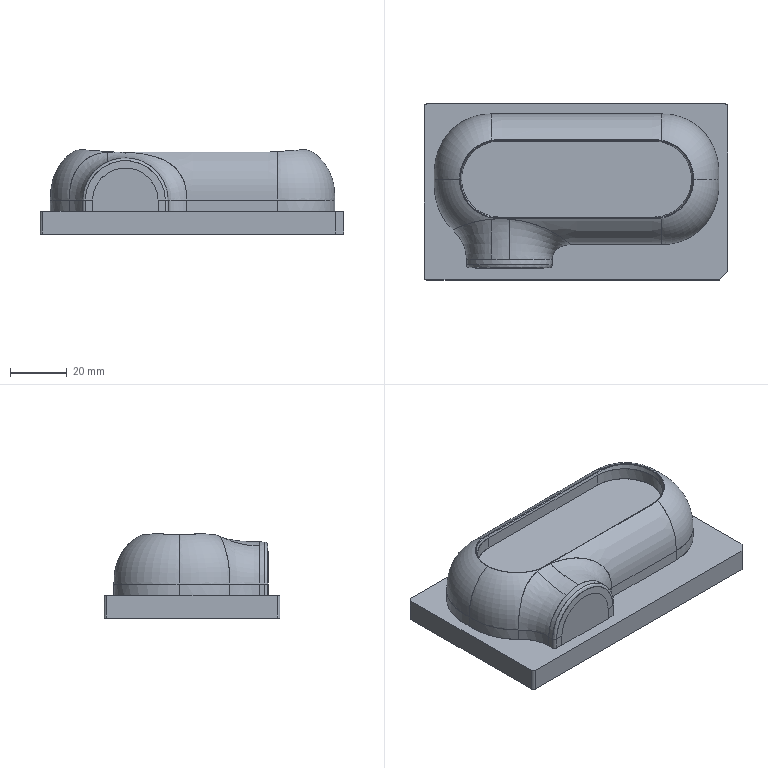NC program | PowerMill | posted by the shop | part box 107 x 62 x 29.663 mm
Lines 358780 to 360246 of 415021:
( TOOL ID   D4_j02_1_1 )
( TOOL DIA. 4. TIP RAD 0 LENGTH 61.48 )
( Z = -6.355 )
T14 M6
T13
G91 G28 Z0
G0 G90 G54
M08
S18000 M3
X0 Y0 M8
G43 Z10.802 H14
X-38.217 Y1.377
Z1.042
G1 Z-.158 F1200
X-38.258 Y1.347 F2000
X-38.295 Y1.313
X-38.33 Y1.276
X-38.362 Y1.237
X-38.391 Y1.195
X-38.416 Y1.152
X-38.438 Y1.106
X-38.456 Y1.059
X-38.47 Y1.011
X-38.481 Y.961
X-38.487 Y.911
X-38.49 Y.861
X-38.489 Y.81
X-38.483 Y.76
X-38.474 Y.71
X-38.461 Y.661
X-38.444 Y.614
X-38.423 Y.568
X-38.399 Y.523
X-38.374 Y.486
X-38.332 Y.425
X-38.291 Y.363
X-38.253 Y.3
X-38.216 Y.236
X-38.159 Y.132
X-38.094 Y.005
X-38.045 Y-.093
X-37.959 Y-.265
X-37.874 Y-.437
X-37.787 Y-.608
X-37.698 Y-.779
X-37.608 Y-.948
X-37.49 Y-1.165
X-37.369 Y-1.379
X-37.245 Y-1.591
X-37.124 Y-1.79
X-37. Y-1.987
X-36.874 Y-2.183
X-36.744 Y-2.377
X-36.612 Y-2.568
X-36.477 Y-2.758
X-36.312 Y-2.986
X-36.144 Y-3.213
X-36.081 Y-3.298
X-35.979 Y-3.436
X-35.905 Y-3.541
X-35.845 Y-3.629
X-35.812 Y-3.681
X-35.78 Y-3.733
X-35.749 Y-3.786
X-35.72 Y-3.84
X-35.704 Y-3.871
X-35.679 Y-3.915
X-35.651 Y-3.957
X-35.619 Y-3.997
X-35.585 Y-4.034
X-35.547 Y-4.068
X-35.507 Y-4.099
X-35.465 Y-4.127
X-35.421 Y-4.151
X-35.375 Y-4.172
X-35.327 Y-4.189
X-35.278 Y-4.202
X-35.229 Y-4.211
X-35.179 Y-4.217
X-35.128 Y-4.218
X-35.078 Y-4.216
X-35.027 Y-4.209
X-34.978 Y-4.199
X-34.93 Y-4.185
X-34.882 Y-4.167
X-34.842 Y-4.147
X-34.039 Y-4.786 Z-.198
X-34.082 Y-4.811
X-34.128 Y-4.834
X-34.175 Y-4.853
X-34.223 Y-4.867
X-34.272 Y-4.879
X-34.322 Y-4.886
X-34.373 Y-4.889
X-34.423 Y-4.888
X-34.473 Y-4.883
X-34.523 Y-4.874
X-34.572 Y-4.862
X-34.62 Y-4.845
X-34.666 Y-4.825
X-34.711 Y-4.801
X-34.753 Y-4.774
X-34.794 Y-4.744
X-34.831 Y-4.71
X-34.866 Y-4.674
X-34.898 Y-4.635
X-34.924 Y-4.598
X-34.965 Y-4.534
X-35.019 Y-4.459
X-35.09 Y-4.363
X-35.168 Y-4.264
X-35.26 Y-4.153
X-35.338 Y-4.062
X-35.478 Y-3.9
X-35.618 Y-3.737
X-35.758 Y-3.573
X-35.896 Y-3.409
X-36.033 Y-3.243
X-36.167 Y-3.075
X-36.306 Y-2.896
X-36.442 Y-2.715
X-36.578 Y-2.528
X-36.711 Y-2.338
X-36.84 Y-2.148
X-36.963 Y-1.959
X-37.083 Y-1.767
X-37.201 Y-1.574
X-37.307 Y-1.391
X-37.411 Y-1.207
X-37.511 Y-1.021
X-37.609 Y-.834
X-37.704 Y-.646
X-37.783 Y-.482
X-37.86 Y-.316
X-37.935 Y-.15
X-38.009 Y.017
X-38.08 Y.184
X-38.155 Y.364
X-38.227 Y.544
X-38.298 Y.725
X-38.368 Y.906
X-38.437 Y1.088
X-38.484 Y1.21
X-38.511 Y1.28
X-38.539 Y1.348
X-38.568 Y1.417
X-38.599 Y1.485
X-38.646 Y1.586
X-38.686 Y1.666
X-38.723 Y1.732
X-38.745 Y1.777
X-38.765 Y1.824
X-38.78 Y1.872
X-38.791 Y1.921
X-38.799 Y1.971
X-38.803 Y2.022
X-38.802 Y2.072
X-38.798 Y2.123
X-38.79 Y2.173
X-38.778 Y2.222
X-38.762 Y2.269
X-38.742 Y2.316
X-38.718 Y2.361
X-38.692 Y2.404
X-38.661 Y2.444
X-38.628 Y2.482
X-38.592 Y2.518
X-38.553 Y2.55
X-38.512 Y2.579
X-38.474 Y2.602
X-38.585 Y3.622 Z-.238
X-38.63 Y3.6
X-38.674 Y3.574
X-38.715 Y3.544
X-38.754 Y3.512
X-38.79 Y3.476
X-38.823 Y3.438
X-38.853 Y3.398
X-38.88 Y3.355
X-38.903 Y3.31
X-38.922 Y3.263
X-38.938 Y3.215
X-38.95 Y3.166
X-38.959 Y3.116
X-38.963 Y3.066
Y3.015
X-38.959 Y2.965
X-38.951 Y2.915
X-38.94 Y2.866
X-38.924 Y2.818
X-38.907 Y2.776
X-38.874 Y2.703
X-38.84 Y2.617
X-38.8 Y2.509
X-38.771 Y2.425
X-38.738 Y2.32
X-38.707 Y2.219
X-38.638 Y1.981
X-38.569 Y1.743
X-38.498 Y1.505
X-38.439 Y1.314
X-38.378 Y1.123
X-38.315 Y.934
X-38.249 Y.745
X-38.169 Y.526
X-38.098 Y.339
X-38.024 Y.153
X-37.948 Y-.031
X-37.868 Y-.215
X-37.771 Y-.43
X-37.683 Y-.616
X-37.592 Y-.802
X-37.491 Y-.997
X-37.389 Y-1.188
X-37.282 Y-1.38
X-37.171 Y-1.571
X-37.058 Y-1.759
X-36.942 Y-1.943
X-36.822 Y-2.125
X-36.714 Y-2.285
X-36.603 Y-2.444
X-36.49 Y-2.601
X-36.374 Y-2.756
X-36.255 Y-2.909
X-36.135 Y-3.061
X-35.997 Y-3.23
X-35.846 Y-3.407
X-35.689 Y-3.587
X-35.529 Y-3.765
X-35.364 Y-3.943
X-35.199 Y-4.117
X-35.049 Y-4.271
X-34.899 Y-4.426
X-34.749 Y-4.581
X-34.657 Y-4.678
X-34.594 Y-4.745
X-34.532 Y-4.812
X-34.471 Y-4.881
X-34.413 Y-4.952
X-34.357 Y-5.025
X-34.312 Y-5.084
X-34.28 Y-5.123
X-34.245 Y-5.16
X-34.207 Y-5.193
X-34.167 Y-5.223
X-34.124 Y-5.251
X-34.079 Y-5.274
X-34.033 Y-5.294
X-33.985 Y-5.311
X-33.936 Y-5.323
X-33.886 Y-5.332
X-33.836 Y-5.336
X-33.785 Y-5.337
X-33.735 Y-5.334
X-33.685 Y-5.326
X-33.636 Y-5.315
X-33.587 Y-5.3
X-33.541 Y-5.281
X-33.495 Y-5.259
X-33.452 Y-5.233
X-33.415 Y-5.207
X-32.881 Y-5.54 Z-.278
X-32.921 Y-5.57
X-32.963 Y-5.598
X-33.008 Y-5.622
X-33.054 Y-5.642
X-33.102 Y-5.658
X-33.151 Y-5.671
X-33.201 Y-5.68
X-33.251 Y-5.685
X-33.302 Y-5.686
X-33.352 Y-5.682
X-33.402 Y-5.675
X-33.451 Y-5.664
X-33.5 Y-5.65
X-33.547 Y-5.631
X-33.592 Y-5.609
X-33.636 Y-5.583
X-33.677 Y-5.554
X-33.716 Y-5.521
X-33.752 Y-5.486
X-33.782 Y-5.452
X-33.85 Y-5.369
X-33.915 Y-5.296
X-33.989 Y-5.217
X-34.068 Y-5.139
X-34.163 Y-5.047
X-34.259 Y-4.956
X-34.436 Y-4.792
X-34.613 Y-4.628
X-34.827 Y-4.427
X-35.001 Y-4.26
X-35.173 Y-4.091
X-35.322 Y-3.94
X-35.469 Y-3.787
X-35.613 Y-3.632
X-35.755 Y-3.475
X-35.895 Y-3.316
X-36.032 Y-3.154
X-36.174 Y-2.982
X-36.312 Y-2.807
X-36.446 Y-2.631
X-36.576 Y-2.452
X-36.703 Y-2.273
X-36.826 Y-2.092
X-36.945 Y-1.909
X-37.061 Y-1.725
X-37.172 Y-1.539
X-37.281 Y-1.351
X-37.386 Y-1.16
X-37.489 Y-.966
X-37.588 Y-.769
X-37.685 Y-.569
X-37.779 Y-.366
X-37.863 Y-.175
X-37.941 Y.011
X-38.016 Y.198
X-38.088 Y.386
X-38.165 Y.596
X-38.232 Y.786
X-38.295 Y.977
X-38.356 Y1.17
X-38.413 Y1.363
X-38.475 Y1.582
X-38.532 Y1.793
X-38.579 Y1.98
X-38.624 Y2.167
X-38.667 Y2.354
X-38.708 Y2.542
X-38.747 Y2.731
X-38.786 Y2.919
X-38.825 Y3.108
X-38.862 Y3.288
X-38.871 Y3.329
X-38.881 Y3.37
X-38.892 Y3.413
X-38.902 Y3.454
X-38.912 Y3.495
X-38.922 Y3.535
X-38.945 Y3.619
X-38.973 Y3.705
X-38.999 Y3.775
X-39.014 Y3.823
X-39.026 Y3.873
X-39.034 Y3.922
X-39.038 Y3.973
Y4.023
X-39.033 Y4.074
X-39.025 Y4.124
X-39.013 Y4.173
X-38.997 Y4.221
X-38.978 Y4.267
X-38.955 Y4.312
X-38.928 Y4.355
X-38.898 Y4.396
X-38.865 Y4.434
X-38.829 Y4.47
X-38.79 Y4.502
X-38.749 Y4.531
X-38.706 Y4.557
X-38.661 Y4.58
X-38.619 Y4.597
G0 Z2.872
G1 X-38.228 Y7.619 F10000
G0 Z1.042
G1 Z-.158 F1200
X-38.268 Y7.65 F2000
X-38.305 Y7.684
X-38.339 Y7.721
X-38.371 Y7.761
X-38.399 Y7.803
X-38.424 Y7.847
X-38.446 Y7.893
X-38.463 Y7.94
X-38.477 Y7.988
X-38.487 Y8.038
X-38.493 Y8.088
X-38.495 Y8.139
X-38.493 Y8.189
X-38.488 Y8.239
X-38.478 Y8.289
X-38.464 Y8.338
X-38.447 Y8.385
X-38.425 Y8.431
X-38.401 Y8.475
X-38.376 Y8.512
X-38.337 Y8.566
X-38.295 Y8.631
X-38.245 Y8.714
X-38.194 Y8.803
X-38.141 Y8.902
X-38.094 Y8.993
X-37.996 Y9.19
X-37.898 Y9.387
X-37.802 Y9.577
X-37.705 Y9.765
X-37.607 Y9.953
X-37.505 Y10.139
X-37.379 Y10.362
X-37.253 Y10.578
X-37.127 Y10.786
X-37. Y10.987
X-36.863 Y11.199
X-36.722 Y11.408
X-36.579 Y11.616
X-36.432 Y11.821
X-36.265 Y12.05
X-36.096 Y12.278
X-36.035 Y12.361
X-35.946 Y12.483
X-35.879 Y12.578
X-35.839 Y12.639
X-35.805 Y12.693
X-35.771 Y12.747
X-35.74 Y12.802
X-35.711 Y12.858
X-35.701 Y12.878
X-35.676 Y12.922
X-35.648 Y12.964
X-35.616 Y13.004
X-35.582 Y13.041
X-35.545 Y13.075
X-35.505 Y13.106
X-35.463 Y13.134
X-35.419 Y13.158
X-35.373 Y13.179
X-35.325 Y13.197
X-35.277 Y13.21
X-35.227 Y13.22
X-35.177 Y13.225
X-35.126 Y13.227
X-35.076 Y13.225
X-35.026 Y13.218
X-34.976 Y13.208
X-34.928 Y13.194
X-34.88 Y13.176
X-34.84 Y13.157
X-34.034 Y13.78 Z-.198
X-34.077 Y13.806
X-34.122 Y13.829
X-34.169 Y13.848
X-34.217 Y13.864
X-34.266 Y13.875
X-34.316 Y13.883
X-34.366 Y13.887
X-34.417 Y13.886
X-34.467 Y13.882
X-34.517 Y13.874
X-34.566 Y13.862
X-34.614 Y13.846
X-34.661 Y13.827
X-34.706 Y13.803
X-34.749 Y13.777
X-34.789 Y13.746
X-34.827 Y13.713
X-34.863 Y13.677
X-34.895 Y13.639
X-34.921 Y13.602
X-34.977 Y13.519
X-35.049 Y13.416
X-35.116 Y13.328
X-35.178 Y13.251
X-35.241 Y13.178
X-35.336 Y13.065
X-35.416 Y12.971
X-35.55 Y12.817
X-35.647 Y12.704
X-35.743 Y12.59
X-35.839 Y12.477
X-35.934 Y12.362
X-36.029 Y12.248
X-36.122 Y12.132
X-36.259 Y11.956
X-36.394 Y11.779
X-36.526 Y11.6
X-36.655 Y11.419
X-36.778 Y11.241
X-36.897 Y11.061
X-37.014 Y10.879
X-37.127 Y10.695
X-37.238 Y10.51
X-37.351 Y10.314
X-37.462 Y10.114
X-37.569 Y9.911
X-37.674 Y9.705
X-37.776 Y9.496
X-37.875 Y9.284
X-37.969 Y9.074
X-38.05 Y8.888
X-38.119 Y8.723
X-38.186 Y8.558
X-38.252 Y8.392
X-38.308 Y8.248
X-38.363 Y8.104
X-38.418 Y7.96
X-38.474 Y7.816
X-38.531 Y7.673
X-38.578 Y7.56
X-38.615 Y7.478
X-38.66 Y7.387
X-38.718 Y7.276
X-38.722 Y7.268
X-38.744 Y7.223
X-38.763 Y7.176
X-38.778 Y7.128
X-38.789 Y7.078
X-38.796 Y7.028
X-38.799 Y6.978
X-38.798 Y6.927
X-38.793 Y6.877
X-38.784 Y6.827
X-38.771 Y6.778
X-38.755 Y6.731
X-38.734 Y6.684
X-38.71 Y6.64
X-38.683 Y6.597
X-38.652 Y6.557
X-38.619 Y6.52
X-38.582 Y6.485
X-38.543 Y6.453
X-38.501 Y6.424
X-38.463 Y6.401
X-38.583 Y5.381 Z-.238
X-38.628 Y5.403
X-38.672 Y5.429
X-38.713 Y5.458
X-38.752 Y5.491
X-38.788 Y5.526
X-38.821 Y5.564
X-38.851 Y5.605
X-38.878 Y5.647
X-38.901 Y5.692
X-38.921 Y5.739
X-38.937 Y5.787
X-38.949 Y5.836
X-38.957 Y5.886
X-38.961 Y5.936
X-38.962 Y5.987
X-38.958 Y6.037
X-38.95 Y6.087
X-38.939 Y6.136
X-38.923 Y6.184
X-38.906 Y6.226
X-38.875 Y6.297
X-38.845 Y6.368
X-38.817 Y6.44
X-38.792 Y6.513
X-38.768 Y6.587
X-38.744 Y6.661
X-38.721 Y6.735
X-38.68 Y6.875
X-38.627 Y7.059
X-38.568 Y7.26
X-38.509 Y7.46
X-38.447 Y7.66
X-38.384 Y7.86
X-38.317 Y8.058
X-38.249 Y8.256
X-38.169 Y8.473
X-38.086 Y8.692
X-37.999 Y8.908
X-37.909 Y9.122
X-37.816 Y9.332
X-37.72 Y9.539
X-37.621 Y9.744
X-37.521 Y9.94
X-37.418 Y10.136
X-37.309 Y10.332
X-37.196 Y10.529
X-37.086 Y10.713
X-36.971 Y10.898
X-36.85 Y11.083
X-36.724 Y11.27
X-36.593 Y11.457
X-36.462 Y11.638
X-36.327 Y11.816
X-36.189 Y11.993
X-36.052 Y12.163
X-35.912 Y12.33
X-35.77 Y12.496
X-35.625 Y12.659
X-35.463 Y12.836
X-35.299 Y13.011
X-35.109 Y13.209
X-34.942 Y13.382
X-34.817 Y13.51
X-34.728 Y13.602
X-34.611 Y13.725
X-34.518 Y13.828
X-34.462 Y13.891
X-34.407 Y13.959
X-34.34 Y14.047
X-34.313 Y14.083
X-34.281 Y14.122
X-34.246 Y14.159
X-34.208 Y14.193
X-34.168 Y14.223
X-34.126 Y14.251
X-34.081 Y14.274
X-34.035 Y14.295
X-33.987 Y14.311
X-33.938 Y14.324
X-33.888 Y14.333
X-33.838 Y14.338
X-33.788 Y14.339
X-33.737 Y14.336
X-33.687 Y14.329
X-33.638 Y14.318
X-33.59 Y14.303
X-33.543 Y14.285
X-33.497 Y14.263
X-33.454 Y14.237
X-33.417 Y14.211
X-32.88 Y14.562 Z-.278
X-32.921 Y14.591
X-32.964 Y14.618
X-33.009 Y14.641
X-33.056 Y14.66
X-33.104 Y14.676
X-33.153 Y14.687
X-33.203 Y14.695
X-33.253 Y14.699
X-33.304
X-33.354 Y14.695
X-33.404 Y14.686
X-33.453 Y14.674
X-33.501 Y14.659
X-33.548 Y14.639
X-33.593 Y14.616
X-33.636 Y14.589
X-33.676 Y14.559
X-33.715 Y14.526
X-33.75 Y14.49
X-33.779 Y14.456
X-33.816 Y14.409
X-33.855 Y14.364
X-33.898 Y14.315
X-33.954 Y14.254
X-33.996 Y14.211
X-34.037 Y14.168
X-34.08 Y14.126
X-34.179 Y14.031
X-34.279 Y13.937
X-34.38 Y13.844
X-34.481 Y13.75
X-34.582 Y13.657
X-34.73 Y13.518
X-34.832 Y13.422
X-35.017 Y13.244
X-35.2 Y13.063
X-35.372 Y12.888
X-35.533 Y12.718
X-35.688 Y12.55
X-35.829 Y12.392
X-35.969 Y12.229
X-36.104 Y12.067
X-36.236 Y11.903
X-36.368 Y11.734
X-36.499 Y11.559
X-36.628 Y11.38
X-36.754 Y11.199
X-36.874 Y11.019
X-36.989 Y10.84
X-37.1 Y10.66
X-37.207 Y10.479
X-37.316 Y10.288
X-37.422 Y10.093
X-37.52 Y9.905
X-37.615 Y9.716
X-37.707 Y9.523
X-37.797 Y9.324
X-37.887 Y9.119
X-37.973 Y8.91
X-38.056 Y8.7
X-38.134 Y8.492
X-38.206 Y8.287
X-38.274 Y8.086
X-38.344 Y7.865
X-38.411 Y7.643
X-38.475 Y7.42
X-38.536 Y7.189
X-38.593 Y6.964
X-38.646 Y6.738
X-38.695 Y6.518
X-38.742 Y6.297
X-38.787 Y6.076
X-38.814 Y5.944
X-38.854 Y5.751
X-38.884 Y5.615
X-38.911 Y5.505
X-38.928 Y5.441
X-38.946 Y5.378
X-38.966 Y5.315
X-38.988 Y5.253
X-39. Y5.222
X-39.015 Y5.174
X-39.027 Y5.125
X-39.035 Y5.075
X-39.039 Y5.024
Y4.974
X-39.035 Y4.923
X-39.028 Y4.874
X-39.016 Y4.824
X-39. Y4.776
X-38.981 Y4.73
X-38.958 Y4.685
X-38.931 Y4.642
X-38.901 Y4.601
X-38.868 Y4.563
X-38.833 Y4.527
X-38.794 Y4.494
X-38.753 Y4.465
X-38.71 Y4.439
X-38.665 Y4.416
X-38.623 Y4.399
G0 Z2.742
G1 X-32.389 Y14.817 F10000
G0 Z.882
G1 Z-.318 F1200
X-32.428 Y14.849 F2000
X-32.47 Y14.877
X-32.514 Y14.902
X-32.559 Y14.924
X-32.607 Y14.942
X-32.655 Y14.956
X-32.705 Y14.967
X-32.755 Y14.973
X-32.805 Y14.976
X-32.856 Y14.974
X-32.906 Y14.968
X-32.956 Y14.959
X-33.004 Y14.946
X-33.052 Y14.929
X-33.098 Y14.908
X-33.142 Y14.883
X-33.184 Y14.855
X-33.224 Y14.824
X-33.261 Y14.79
X-33.292 Y14.757
X-33.342 Y14.701
X-33.394 Y14.645
X-33.461 Y14.579
X-33.541 Y14.504
X-33.614 Y14.437
X-33.744 Y14.323
X-33.911 Y14.182
X-34.097 Y14.025
X-34.26 Y13.886
X-34.423 Y13.747
X-34.584 Y13.606
X-34.744 Y13.463
X-34.902 Y13.318
X-35.08 Y13.149
X-35.255 Y12.979
X-35.426 Y12.807
X-35.586 Y12.64
X-35.743 Y12.471
X-35.892 Y12.305
X-36.033 Y12.143
X-36.167 Y11.982
X-36.297 Y11.821
X-36.425 Y11.655
X-36.551 Y11.486
X-36.675 Y11.312
X-36.797 Y11.135
X-36.914 Y10.957
X-37.028 Y10.779
X-37.136 Y10.6
X-37.241 Y10.42
X-37.344 Y10.236
X-37.445 Y10.047
X-37.536 Y9.869
X-37.618 Y9.702
X-37.697 Y9.533
X-37.774 Y9.364
X-37.848 Y9.193
X-37.918 Y9.022
X-37.997 Y8.821
X-38.076 Y8.608
X-38.145 Y8.413
X-38.217 Y8.202
X-38.285 Y7.988
X-38.349 Y7.774
X-38.41 Y7.559
X-38.468 Y7.343
X-38.522 Y7.121
X-38.574 Y6.895
X-38.623 Y6.663
X-38.67 Y6.426
X-38.713 Y6.182
X-38.75 Y5.959
X-38.786 Y5.716
X-38.819 Y5.472
X-38.849 Y5.228
X-38.864 Y5.103
X-38.876 Y4.975
X-38.888 Y4.825
X-38.896 Y4.683
X-38.9 Y4.557
X-38.901 Y4.443
X-38.898 Y4.343
X-38.893 Y4.243
X-38.886 Y4.143
X-38.877 Y4.035
X-38.862 Y3.889
X-38.848 Y3.759
X-38.836 Y3.66
X-38.823 Y3.561
X-38.81 Y3.461
X-38.797 Y3.362
X-38.761 Y3.114
X-38.728 Y2.902
X-38.687 Y2.666
X-38.641 Y2.426
X-38.594 Y2.195
X-38.543 Y1.966
X-38.491 Y1.752
X-38.433 Y1.525
X-38.372 Y1.305
X-38.309 Y1.089
X-38.243 Y.88
X-38.175 Y.673
X-38.094 Y.442
X-38.015 Y.228
X-37.938 Y.028
X-37.862 Y-.16
X-37.782 Y-.346
X-37.697 Y-.534
X-37.608 Y-.724
X-37.512 Y-.916
X-37.414 Y-1.106
X-37.315 Y-1.29
X-37.213 Y-1.468
X-37.11 Y-1.644
X-37.003 Y-1.817
X-36.894 Y-1.989
X-36.781 Y-2.159
X-36.665 Y-2.326
X-36.546 Y-2.492
X-36.427 Y-2.652
X-36.305 Y-2.81
X-36.172 Y-2.976
X-36.059 Y-3.113
X-35.941 Y-3.25
X-35.807 Y-3.4
X-35.648 Y-3.573
X-35.526 Y-3.702
X-35.379 Y-3.855
X-35.229 Y-4.005
X-35.077 Y-4.153
X-34.923 Y-4.299
X-34.767 Y-4.442
X-34.609 Y-4.584
X-34.39 Y-4.776
X-34.189 Y-4.947
X-33.987 Y-5.118
X-33.825 Y-5.255
X-33.685 Y-5.375
X-33.585 Y-5.463
X-33.495 Y-5.547
X-33.417 Y-5.622
X-33.354 Y-5.688
X-33.301 Y-5.747
X-33.294 Y-5.756
X-33.259 Y-5.793
X-33.222 Y-5.827
X-33.183 Y-5.859
X-33.141 Y-5.887
X-33.097 Y-5.912
X-33.051 Y-5.933
X-33.004 Y-5.951
X-32.955 Y-5.965
X-32.906 Y-5.974
X-32.855 Y-5.98
X-32.805 Y-5.982
X-32.754 Y-5.98
X-32.704 Y-5.974
X-32.655 Y-5.965
X-32.606 Y-5.951
X-32.559 Y-5.933
X-32.513 Y-5.912
X-32.469 Y-5.887
X-32.427 Y-5.859
X-32.392 Y-5.831
X-31.925 Y-6.039 Z-.358
X-31.963 Y-6.072
X-32.004 Y-6.102
X-32.046 Y-6.129
X-32.091 Y-6.153
X-32.137 Y-6.173
X-32.185 Y-6.189
X-32.234 Y-6.201
X-32.284 Y-6.21
X-32.334 Y-6.214
X-32.385 Y-6.215
X-32.435 Y-6.211
X-32.485 Y-6.204
X-32.535 Y-6.193
X-32.583 Y-6.177
X-32.63 Y-6.158
X-32.675 Y-6.136
X-32.718 Y-6.11
X-32.759 Y-6.08
X-32.798 Y-6.048
X-32.83 Y-6.016
X-32.871 Y-5.973
X-32.914 Y-5.931
X-32.963 Y-5.885
X-33.023 Y-5.832
X-33.068 Y-5.792
X-33.113 Y-5.754
X-33.23 Y-5.657
X-33.37 Y-5.546
X-33.547 Y-5.409
X-33.74 Y-5.26
X-33.933 Y-5.11
X-34.123 Y-4.959
X-34.313 Y-4.805
X-34.466 Y-4.678
X-34.617 Y-4.548
X-34.766 Y-4.417
X-34.915 Y-4.285
X-35.062 Y-4.151
X-35.222 Y-4.002
X-35.373 Y-3.855
X-35.517 Y-3.71
X-35.655 Y-3.566
X-35.802 Y-3.406
X-35.944 Y-3.246
X-36.08 Y-3.087
X-36.211 Y-2.928
X-36.338 Y-2.768
X-36.463 Y-2.604
X-36.586 Y-2.437
X-36.707 Y-2.267
X-36.824 Y-2.094
X-36.938 Y-1.921
X-37.048 Y-1.746
X-37.155 Y-1.568
X-37.261 Y-1.385
X-37.364 Y-1.2
X-37.463 Y-1.013
X-37.559 Y-.823
X-37.652 Y-.632
X-37.741 Y-.438
X-37.827 Y-.241
X-37.91 Y-.043
X-37.984 Y.146
X-38.057 Y.341
X-38.13 Y.547
X-38.192 Y.73
X-38.25 Y.915
X-38.306 Y1.104
X-38.363 Y1.31
X-38.421 Y1.533
X-38.477 Y1.761
X-38.525 Y1.974
X-38.566 Y2.163
X-38.606 Y2.365
X-38.642 Y2.567
X-38.677 Y2.774
X-38.708 Y2.977
X-38.734 Y3.173
X-38.759 Y3.379
X-38.783 Y3.601
X-38.801 Y3.796
X-38.814 Y3.981
X-38.823 Y4.146
X-38.829 Y4.312
X-38.831 Y4.477
X-38.83 Y4.643
X-38.825 Y4.818
X-38.816 Y4.986
X-38.805 Y5.152
X-38.791 Y5.317
X-38.774 Y5.482
X-38.756 Y5.646
X-38.733 Y5.836
X-38.708 Y6.025
X-38.679 Y6.214
X-38.647 Y6.402
X-38.614 Y6.59
X-38.575 Y6.793
X-38.532 Y6.996
X-38.486 Y7.198
X-38.441 Y7.387
X-38.393 Y7.576
X-38.343 Y7.764
X-38.29 Y7.952
X-38.234 Y8.138
X-38.174 Y8.323
X-38.112 Y8.508
X-38.039 Y8.709
X-37.963 Y8.909
X-37.883 Y9.108
X-37.8 Y9.305
X-37.713 Y9.5
X-37.622 Y9.694
X-37.527 Y9.886
X-37.429 Y10.078
X-37.328 Y10.265
X-37.225 Y10.448
X-37.12 Y10.627
X-37.008 Y10.81
X-36.893 Y10.99
X-36.775 Y11.168
X-36.653 Y11.343
X-36.528 Y11.516
X-36.401 Y11.687
X-36.27 Y11.855
X-36.136 Y12.02
X-35.999 Y12.183
X-35.859 Y12.343
X-35.716 Y12.5
X-35.571 Y12.654
X-35.423 Y12.805
X-35.273 Y12.953
X-35.12 Y13.098
X-34.964 Y13.24
X-34.769 Y13.416
X-34.601 Y13.563
X-34.444 Y13.697
X-34.26 Y13.848
X-34.061 Y14.009
X-33.845 Y14.178
X-33.663 Y14.32
X-33.428 Y14.501
X-33.271 Y14.624
X-33.148 Y14.724
X-33.046 Y14.811
X-32.958 Y14.89
X-32.879 Y14.965
X-32.829 Y15.016
X-32.792 Y15.051
X-32.753 Y15.083
X-32.711 Y15.111
X-32.667 Y15.136
X-32.622 Y15.158
X-32.574 Y15.176
X-32.526 Y15.19
X-32.476 Y15.2
X-32.426 Y15.206
X-32.376 Y15.208
X-32.325 Y15.206
X-32.275 Y15.201
X-32.225 Y15.191
X-32.177 Y15.177
X-32.129 Y15.16
X-32.083 Y15.139
X-32.039 Y15.114
X-31.997 Y15.086
X-31.957 Y15.055
X-31.924 Y15.025
X-31.487 Y15.202 Z-.398
X-31.522 Y15.238
X-31.561 Y15.27
X-31.602 Y15.3
X-31.645 Y15.326
X-31.69 Y15.349
X-31.737 Y15.369
X-31.785 Y15.384
X-31.834 Y15.396
X-31.884 Y15.403
X-31.934 Y15.407
X-31.985
X-32.035 Y15.403
X-32.085 Y15.394
X-32.134 Y15.382
X-32.182 Y15.366
X-32.229 Y15.347
X-32.274 Y15.324
X-32.316 Y15.297
X-32.357 Y15.267
X-32.391 Y15.237
X-32.477 Y15.158
X-32.566 Y15.081
X-32.662 Y15.003
X-32.765 Y14.923
X-32.86 Y14.854
X-33.083 Y14.693
X-33.308 Y14.533
X-33.532 Y14.373
X-33.755 Y14.211
X-33.92 Y14.089
X-34.083 Y13.964
X-34.245 Y13.837
X-34.406 Y13.71
X-34.565 Y13.581
X-34.723 Y13.451
X-34.878 Y13.317
X-35.031 Y13.18
X-35.181 Y13.041
X-35.334 Y12.894
X-35.484 Y12.744
X-35.63 Y12.593
X-35.773 Y12.439
X-35.912 Y12.283
X-36.033 Y12.143
X-36.151 Y12.
X-36.266 Y11.856
X-36.379 Y11.71
X-36.507 Y11.538
X-36.616 Y11.388
X-36.721 Y11.237
X-36.84 Y11.061
X-36.959 Y10.877
X-37.072 Y10.695
X-37.183 Y10.511
X-37.29 Y10.323
X-37.395 Y10.133
X-37.496 Y9.939
X-37.595 Y9.744
X-37.687 Y9.551
X-37.774 Y9.362
X-37.855 Y9.175
X-37.931 Y8.991
X-38.003 Y8.806
X-38.077 Y8.605
X-38.148 Y8.402
X-38.212 Y8.208
X-38.272 Y8.013
X-38.329 Y7.816
X-38.382 Y7.619
X-38.434 Y7.415
X-38.48 Y7.216
X-38.516 Y7.048
X-38.55 Y6.881
X-38.581 Y6.712
X-38.61 Y6.544
X-38.638 Y6.365
X-38.664 Y6.196
X-38.688 Y6.027
X-38.709 Y5.857
X-38.729 Y5.687
X-38.748 Y5.497
X-38.764 Y5.306
X-38.778 Y5.105
X-38.788 Y4.906
X-38.794 Y4.715
X-38.797 Y4.524
X-38.795 Y4.333
X-38.79 Y4.143
X-38.781 Y3.947
X-38.768 Y3.741
X-38.75 Y3.527
X-38.728 Y3.307
X-38.709 Y3.143
X-38.689 Y2.978
X-38.666 Y2.814
X-38.641 Y2.65
X-38.615 Y2.486
X-38.588 Y2.322
X-38.55 Y2.117
X-38.508 Y1.909
X-38.461 Y1.7
X-38.41 Y1.49
X-38.355 Y1.278
X-38.301 Y1.084
X-38.243 Y.891
X-38.182 Y.699
X-38.116 Y.505
X-38.044 Y.304
X-37.973 Y.116
X-37.898 Y-.071
X-37.829 Y-.237
X-37.756 Y-.401
X-37.681 Y-.564
X-37.598 Y-.736
X-37.518 Y-.897
X-37.435 Y-1.056
X-37.35 Y-1.215
X-37.246 Y-1.401
X-37.152 Y-1.563
X-37.035 Y-1.755
X-36.917 Y-1.942
X-36.798 Y-2.125
X-36.676 Y-2.303
X-36.553 Y-2.477
X-36.433 Y-2.638
X-36.3 Y-2.813
X-36.173 Y-2.973
X-36.052 Y-3.12
X-35.932 Y-3.26
X-35.791 Y-3.419
X-35.646 Y-3.575
X-35.499 Y-3.728
X-35.35 Y-3.878
X-35.197 Y-4.025
X-35.042 Y-4.17
X-34.884 Y-4.312
X-34.723 Y-4.451
X-34.559 Y-4.587
X-34.396 Y-4.718
X-34.232 Y-4.848
X-34.067 Y-4.977
X-33.9 Y-5.103
X-33.749 Y-5.216
X-33.596 Y-5.327
X-33.442 Y-5.437
X-33.289 Y-5.547
X-33.135 Y-5.656
X-32.951 Y-5.788
X-32.855 Y-5.857
X-32.768 Y-5.921
X-32.683 Y-5.987
X-32.598 Y-6.054
X-32.514 Y-6.125
X-32.434 Y-6.197
X-32.392 Y-6.236
X-32.354 Y-6.269
X-32.313 Y-6.299
X-32.27 Y-6.326
X-32.226 Y-6.349
X-32.179 Y-6.369
X-32.131 Y-6.384
X-32.082 Y-6.396
X-32.032 Y-6.405
X-31.982 Y-6.409
X-31.931
X-31.881 Y-6.405
X-31.831 Y-6.397
X-31.782 Y-6.385
X-31.734 Y-6.37
X-31.687 Y-6.35
X-31.642 Y-6.327
X-31.599 Y-6.301
X-31.558 Y-6.271
X-31.52 Y-6.238
X-31.488 Y-6.207
X-31.069 Y-6.361 Z-.438
X-31.103 Y-6.398
X-31.14 Y-6.432
X-31.18 Y-6.463
X-31.222 Y-6.491
X-31.267 Y-6.515
X-31.313 Y-6.536
X-31.36 Y-6.553
X-31.409 Y-6.566
X-31.459 Y-6.576
X-31.509 Y-6.581
X-31.559 Y-6.583
X-31.61 Y-6.58
X-31.66 Y-6.574
X-31.709 Y-6.564
X-31.758 Y-6.549
X-31.805 Y-6.531
X-31.851 Y-6.51
X-31.894 Y-6.485
X-31.936 Y-6.456
X-31.971 Y-6.428
X-32.052 Y-6.358
X-32.135 Y-6.291
X-32.22 Y-6.226
X-32.311 Y-6.16
X-32.399 Y-6.099
X-32.488 Y-6.039
X-32.654 Y-5.928
X-32.822 Y-5.819
X-32.99 Y-5.709
X-33.164 Y-5.594
X-33.337 Y-5.478
X-33.51 Y-5.36
X-33.682 Y-5.241
X-33.792 Y-5.163
X-33.903 Y-5.084
X-34.013 Y-5.005
X-34.123 Y-4.925
X-34.232 Y-4.844
X-34.339 Y-4.761
X-34.446 Y-4.678
X-34.605 Y-4.549
X-34.761 Y-4.418
X-34.916 Y-4.283
X-35.067 Y-4.147
X-35.179 Y-4.043
X-35.288 Y-3.938
X-35.395 Y-3.83
X-35.5 Y-3.721
X-35.617 Y-3.598
X-35.719 Y-3.486
X-35.821 Y-3.373
X-35.921 Y-3.259
X-36.055 Y-3.1
X-36.187 Y-2.938
X-36.323 Y-2.766
X-36.449 Y-2.6
X-36.572 Y-2.432
X-36.692 Y-2.261
X-36.814 Y-2.08
X-36.933 Y-1.897
X-37.049 Y-1.712
X-37.162 Y-1.524
X-37.271 Y-1.335
X-37.377 Y-1.144
X-37.475 Y-.957
X-37.571 Y-.768
X-37.663 Y-.577
X-37.751 Y-.385
X-37.835 Y-.196
X-37.915 Y-.005
X-37.992 Y.187
X-38.066 Y.382
X-38.136 Y.577
X-38.2 Y.764
X-38.26 Y.952
X-38.317 Y1.142
X-38.37 Y1.335
X-38.421 Y1.534
X-38.47 Y1.738
X-38.515 Y1.947
X-38.554 Y2.141
X-38.591 Y2.341
X-38.624 Y2.542
X-38.654 Y2.744
X-38.68 Y2.946
X-38.703 Y3.148
X-38.715 Y3.268
X-38.725 Y3.389
X-38.734 Y3.509
X-38.743 Y3.63
X-38.751 Y3.751
X-38.759 Y3.871
X-38.765 Y3.992
X-38.77 Y4.113
X-38.775 Y4.342
X-38.776 Y4.567
X-38.774 Y4.743
X-38.768 Y4.919
X-38.76 Y5.095
X-38.75 Y5.271
X-38.738 Y5.446
X-38.724 Y5.622
X-38.708 Y5.797
X-38.69 Y5.972
X-38.665 Y6.175
X-38.636 Y6.378
X-38.604 Y6.58
X-38.569 Y6.781
X-38.53 Y6.982
X-38.485 Y7.192
X-38.437 Y7.402
X-38.392 Y7.582
X-38.344 Y7.761
X-38.293 Y7.939
X-38.239 Y8.116
X-38.181 Y8.292
X-38.12 Y8.467
X-38.057 Y8.641
X-37.98 Y8.842
X-37.899 Y9.043
X-37.814 Y9.243
X-37.725 Y9.443
X-37.633 Y9.64
X-37.537 Y9.836
X-37.438 Y10.029
X-37.334 Y10.221
X-37.228 Y10.411
X-37.118 Y10.599
X-37.004 Y10.785
X-36.887 Y10.97
X-36.766 Y11.152
X-36.643 Y11.331
X-36.516 Y11.508
X-36.386 Y11.683
X-36.253 Y11.856
X-36.117 Y12.025
X-35.977 Y12.192
X-35.835 Y12.357
X-35.719 Y12.486
X-35.602 Y12.614
X-35.474 Y12.749
X-35.352 Y12.873
X-35.23 Y12.994
X-35.105 Y13.112
X-34.977 Y13.229
X-34.848 Y13.343
X-34.718 Y13.455
X-34.553 Y13.591
X-34.388 Y13.724
X-34.24 Y13.838
X-34.14 Y13.913
X-34.04 Y13.986
X-33.938 Y14.058
X-33.836 Y14.131
X-33.735 Y14.203
X-33.53 Y14.347
X-33.323 Y14.488
X-33.114 Y14.627
X-32.905 Y14.765
X-32.813 Y14.825
X-32.722 Y14.884
X-32.63 Y14.944
X-32.539 Y15.004
X-32.45 Y15.063
X-32.37 Y15.119
X-32.289 Y15.175
X-32.21 Y15.233
X-32.132 Y15.293
X-32.056 Y15.355
X-31.982 Y15.418
X-31.972 Y15.427
X-31.932 Y15.459
X-31.891 Y15.488
X-31.847 Y15.513
X-31.801 Y15.535
X-31.754 Y15.553
X-31.706 Y15.567
X-31.656 Y15.578
X-31.606 Y15.584
X-31.556 Y15.587
X-31.505 Y15.585
X-31.455 Y15.58
X-31.405 Y15.57
X-31.357 Y15.557
X-31.309 Y15.54
X-31.263 Y15.519
X-31.219 Y15.495
X-31.177 Y15.467
X-31.137 Y15.436
X-31.099 Y15.402
X-31.069 Y15.369
X-30.668 Y15.497 Z-.478
X-30.701 Y15.535
X-30.737 Y15.571
X-30.776 Y15.603
X-30.818 Y15.632
X-30.861 Y15.658
X-30.907 Y15.68
X-30.954 Y15.698
X-31.002 Y15.713
X-31.051 Y15.724
X-31.101 Y15.731
X-31.152 Y15.734
X-31.202 Y15.733
X-31.252 Y15.728
X-31.302 Y15.719
X-31.351 Y15.706
X-31.399 Y15.69
X-31.445 Y15.669
X-31.49 Y15.646
X-31.532 Y15.618
X-31.568 Y15.591
X-31.641 Y15.532
X-31.715 Y15.475
X-31.791 Y15.421
X-31.877 Y15.363
X-31.955 Y15.312
X-32.034 Y15.261
X-32.184 Y15.168
X-32.356 Y15.064
X-32.577 Y14.93
X-32.798 Y14.797
X-33.018 Y14.662
X-33.236 Y14.523
X-33.453 Y14.384
X-33.633 Y14.267
X-33.811 Y14.147
X-33.986 Y14.025
X-34.154 Y13.902
X-34.32 Y13.776
X-34.486 Y13.646
X-34.602 Y13.551
X-34.717 Y13.454
X-34.829 Y13.355
X-34.941 Y13.254
X-35.076 Y13.128
X-35.184 Y13.024